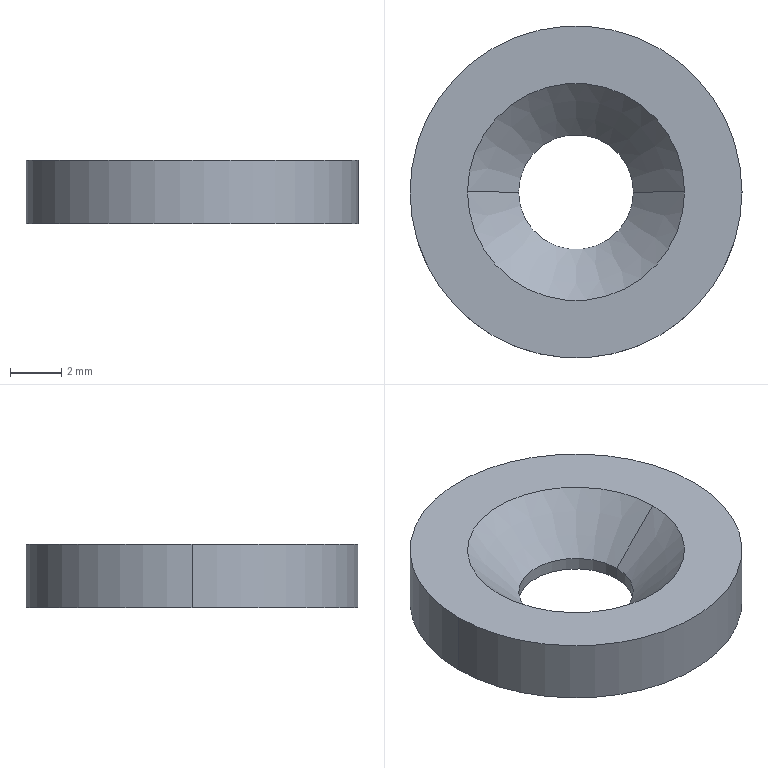Part | NX | features BREP 1 | 1 solid | 8 faces | box 13 x 13 x 2.5 mm | volume 255.418 mm3 | cylinder 4 | cone 2 | plane 2 | commonest cylinder face diameters 4.5 x2 13 x2
STEP:
#1=CARTESIAN_POINT('',(-4.25,0.,2.5));
#2=VERTEX_POINT('',#1);
#3=CARTESIAN_POINT('',(-2.25,0.,0.5));
#4=VERTEX_POINT('',#3);
#5=CARTESIAN_POINT('',(-4.25,0.,2.5));
#6=DIRECTION('',(-0.7071,0.,0.7071));
#7=VECTOR('',#6,1000.);
#8=LINE('',#5,#7);
#9=EDGE_CURVE('',#2,#4,#8,.F.);
#10=ORIENTED_EDGE('',*,*,#9,.T.);
#11=CARTESIAN_POINT('',(2.25,0.,0.5));
#12=VERTEX_POINT('',#11);
#13=CARTESIAN_POINT('',(0.,0.,0.5));
#14=DIRECTION('',(0.,0.,1.));
#15=DIRECTION('',(1.,0.,0.));
#16=AXIS2_PLACEMENT_3D('',#13,#14,#15);
#17=CIRCLE('',#16,2.25);
#18=EDGE_CURVE('',#12,#4,#17,.T.);
#19=ORIENTED_EDGE('',*,*,#18,.F.);
#20=CARTESIAN_POINT('',(4.25,0.,2.5));
#21=VERTEX_POINT('',#20);
#22=CARTESIAN_POINT('',(4.25,0.,2.5));
#23=DIRECTION('',(0.7071,0.,0.7071));
#24=VECTOR('',#23,1000.);
#25=LINE('',#22,#24);
#26=EDGE_CURVE('',#21,#12,#25,.F.);
#27=ORIENTED_EDGE('',*,*,#26,.F.);
#28=CARTESIAN_POINT('',(0.,0.,2.5));
#29=DIRECTION('',(0.,0.,1.));
#30=DIRECTION('',(1.,0.,0.));
#31=AXIS2_PLACEMENT_3D('',#28,#29,#30);
#32=CIRCLE('',#31,4.25);
#33=EDGE_CURVE('',#21,#2,#32,.T.);
#34=ORIENTED_EDGE('',*,*,#33,.T.);
#35=EDGE_LOOP('',(#10,#19,#27,#34));
#36=FACE_BOUND('',#35,.T.);
#37=CARTESIAN_POINT('',(0.,0.,2.5));
#38=DIRECTION('',(0.,0.,1.));
#39=DIRECTION('',(1.,0.,0.));
#40=AXIS2_PLACEMENT_3D('',#37,#38,#39);
#41=CONICAL_SURFACE('',#40,4.25,0.7854);
#42=ADVANCED_FACE('',(#36),#41,.F.);
#43=CARTESIAN_POINT('',(-2.25,0.,0.));
#44=VERTEX_POINT('',#43);
#45=CARTESIAN_POINT('',(-2.25,0.,2.5));
#46=DIRECTION('',(0.,0.,1.));
#47=VECTOR('',#46,1000.);
#48=LINE('',#45,#47);
#49=EDGE_CURVE('',#4,#44,#48,.F.);
#50=ORIENTED_EDGE('',*,*,#49,.T.);
#51=CARTESIAN_POINT('',(2.25,0.,0.));
#52=VERTEX_POINT('',#51);
#53=CARTESIAN_POINT('',(0.,0.,0.));
#54=DIRECTION('',(0.,0.,1.));
#55=DIRECTION('',(1.,0.,0.));
#56=AXIS2_PLACEMENT_3D('',#53,#54,#55);
#57=CIRCLE('',#56,2.25);
#58=EDGE_CURVE('',#52,#44,#57,.T.);
#59=ORIENTED_EDGE('',*,*,#58,.F.);
#60=CARTESIAN_POINT('',(2.25,0.,2.5));
#61=DIRECTION('',(0.,0.,1.));
#62=VECTOR('',#61,1000.);
#63=LINE('',#60,#62);
#64=EDGE_CURVE('',#12,#52,#63,.F.);
#65=ORIENTED_EDGE('',*,*,#64,.F.);
#66=ORIENTED_EDGE('',*,*,#18,.T.);
#67=EDGE_LOOP('',(#50,#59,#65,#66));
#68=FACE_BOUND('',#67,.T.);
#69=CARTESIAN_POINT('',(0.,0.,2.5));
#70=DIRECTION('',(0.,0.,1.));
#71=DIRECTION('',(1.,0.,0.));
#72=AXIS2_PLACEMENT_3D('',#69,#70,#71);
#73=CYLINDRICAL_SURFACE('',#72,2.25);
#74=ADVANCED_FACE('',(#68),#73,.F.);
#75=CARTESIAN_POINT('',(-6.5,0.,0.));
#76=VERTEX_POINT('',#75);
#77=CARTESIAN_POINT('',(6.5,0.,0.));
#78=VERTEX_POINT('',#77);
#79=CARTESIAN_POINT('',(0.,0.,0.));
#80=DIRECTION('',(0.,0.,1.));
#81=DIRECTION('',(1.,0.,0.));
#82=AXIS2_PLACEMENT_3D('',#79,#80,#81);
#83=CIRCLE('',#82,6.5);
#84=EDGE_CURVE('',#76,#78,#83,.T.);
#85=ORIENTED_EDGE('',*,*,#84,.F.);
#86=CARTESIAN_POINT('',(0.,0.,0.));
#87=DIRECTION('',(0.,0.,1.));
#88=DIRECTION('',(1.,0.,0.));
#89=AXIS2_PLACEMENT_3D('',#86,#87,#88);
#90=CIRCLE('',#89,6.5);
#91=EDGE_CURVE('',#78,#76,#90,.T.);
#92=ORIENTED_EDGE('',*,*,#91,.F.);
#93=EDGE_LOOP('',(#85,#92));
#94=FACE_BOUND('',#93,.T.);
#95=ORIENTED_EDGE('',*,*,#58,.T.);
#96=CARTESIAN_POINT('',(0.,0.,0.));
#97=DIRECTION('',(0.,0.,1.));
#98=DIRECTION('',(1.,0.,0.));
#99=AXIS2_PLACEMENT_3D('',#96,#97,#98);
#100=CIRCLE('',#99,2.25);
#101=EDGE_CURVE('',#44,#52,#100,.T.);
#102=ORIENTED_EDGE('',*,*,#101,.T.);
#103=EDGE_LOOP('',(#95,#102));
#104=FACE_BOUND('',#103,.T.);
#105=CARTESIAN_POINT('',(0.,0.,0.));
#106=DIRECTION('',(0.,0.,1.));
#107=DIRECTION('',(1.,0.,0.));
#108=AXIS2_PLACEMENT_3D('',#105,#106,#107);
#109=PLANE('',#108);
#110=ADVANCED_FACE('',(#94,#104),#109,.F.);
#111=CARTESIAN_POINT('',(-6.5,0.,2.5));
#112=VERTEX_POINT('',#111);
#113=CARTESIAN_POINT('',(6.5,0.,2.5));
#114=VERTEX_POINT('',#113);
#115=CARTESIAN_POINT('',(0.,0.,2.5));
#116=DIRECTION('',(0.,0.,1.));
#117=DIRECTION('',(1.,0.,0.));
#118=AXIS2_PLACEMENT_3D('',#115,#116,#117);
#119=CIRCLE('',#118,6.5);
#120=EDGE_CURVE('',#112,#114,#119,.T.);
#121=ORIENTED_EDGE('',*,*,#120,.T.);
#122=CARTESIAN_POINT('',(0.,0.,2.5));
#123=DIRECTION('',(0.,0.,1.));
#124=DIRECTION('',(1.,0.,0.));
#125=AXIS2_PLACEMENT_3D('',#122,#123,#124);
#126=CIRCLE('',#125,6.5);
#127=EDGE_CURVE('',#114,#112,#126,.T.);
#128=ORIENTED_EDGE('',*,*,#127,.T.);
#129=EDGE_LOOP('',(#121,#128));
#130=FACE_BOUND('',#129,.T.);
#131=ORIENTED_EDGE('',*,*,#33,.F.);
#132=CARTESIAN_POINT('',(0.,0.,2.5));
#133=DIRECTION('',(0.,0.,1.));
#134=DIRECTION('',(1.,0.,0.));
#135=AXIS2_PLACEMENT_3D('',#132,#133,#134);
#136=CIRCLE('',#135,4.25);
#137=EDGE_CURVE('',#2,#21,#136,.T.);
#138=ORIENTED_EDGE('',*,*,#137,.F.);
#139=EDGE_LOOP('',(#131,#138));
#140=FACE_BOUND('',#139,.T.);
#141=CARTESIAN_POINT('',(0.,0.,2.5));
#142=DIRECTION('',(0.,0.,1.));
#143=DIRECTION('',(1.,0.,0.));
#144=AXIS2_PLACEMENT_3D('',#141,#142,#143);
#145=PLANE('',#144);
#146=ADVANCED_FACE('',(#130,#140),#145,.T.);
#147=CARTESIAN_POINT('',(6.5,0.,2.5));
#148=DIRECTION('',(0.,0.,-1.));
#149=VECTOR('',#148,1000.);
#150=LINE('',#147,#149);
#151=EDGE_CURVE('',#114,#78,#150,.T.);
#152=ORIENTED_EDGE('',*,*,#151,.F.);
#153=ORIENTED_EDGE('',*,*,#120,.F.);
#154=CARTESIAN_POINT('',(-6.5,0.,2.5));
#155=DIRECTION('',(0.,0.,-1.));
#156=VECTOR('',#155,1000.);
#157=LINE('',#154,#156);
#158=EDGE_CURVE('',#112,#76,#157,.T.);
#159=ORIENTED_EDGE('',*,*,#158,.T.);
#160=ORIENTED_EDGE('',*,*,#84,.T.);
#161=EDGE_LOOP('',(#152,#153,#159,#160));
#162=FACE_BOUND('',#161,.T.);
#163=CARTESIAN_POINT('',(0.,0.,2.5));
#164=DIRECTION('',(0.,0.,-1.));
#165=DIRECTION('',(-1.,0.,0.));
#166=AXIS2_PLACEMENT_3D('',#163,#164,#165);
#167=CYLINDRICAL_SURFACE('',#166,6.5);
#168=ADVANCED_FACE('',(#162),#167,.T.);
#169=ORIENTED_EDGE('',*,*,#127,.F.);
#170=ORIENTED_EDGE('',*,*,#151,.T.);
#171=ORIENTED_EDGE('',*,*,#91,.T.);
#172=ORIENTED_EDGE('',*,*,#158,.F.);
#173=EDGE_LOOP('',(#169,#170,#171,#172));
#174=FACE_BOUND('',#173,.T.);
#175=CARTESIAN_POINT('',(0.,0.,2.5));
#176=DIRECTION('',(0.,0.,-1.));
#177=DIRECTION('',(-1.,0.,0.));
#178=AXIS2_PLACEMENT_3D('',#175,#176,#177);
#179=CYLINDRICAL_SURFACE('',#178,6.5);
#180=ADVANCED_FACE('',(#174),#179,.T.);
#181=ORIENTED_EDGE('',*,*,#101,.F.);
#182=ORIENTED_EDGE('',*,*,#49,.F.);
#183=CARTESIAN_POINT('',(0.,0.,0.5));
#184=DIRECTION('',(0.,0.,1.));
#185=DIRECTION('',(1.,0.,0.));
#186=AXIS2_PLACEMENT_3D('',#183,#184,#185);
#187=CIRCLE('',#186,2.25);
#188=EDGE_CURVE('',#4,#12,#187,.T.);
#189=ORIENTED_EDGE('',*,*,#188,.T.);
#190=ORIENTED_EDGE('',*,*,#64,.T.);
#191=EDGE_LOOP('',(#181,#182,#189,#190));
#192=FACE_BOUND('',#191,.T.);
#193=CARTESIAN_POINT('',(0.,0.,2.5));
#194=DIRECTION('',(0.,0.,1.));
#195=DIRECTION('',(1.,0.,0.));
#196=AXIS2_PLACEMENT_3D('',#193,#194,#195);
#197=CYLINDRICAL_SURFACE('',#196,2.25);
#198=ADVANCED_FACE('',(#192),#197,.F.);
#199=ORIENTED_EDGE('',*,*,#188,.F.);
#200=ORIENTED_EDGE('',*,*,#9,.F.);
#201=ORIENTED_EDGE('',*,*,#137,.T.);
#202=ORIENTED_EDGE('',*,*,#26,.T.);
#203=EDGE_LOOP('',(#199,#200,#201,#202));
#204=FACE_BOUND('',#203,.T.);
#205=CARTESIAN_POINT('',(0.,0.,2.5));
#206=DIRECTION('',(0.,0.,1.));
#207=DIRECTION('',(1.,0.,0.));
#208=AXIS2_PLACEMENT_3D('',#205,#206,#207);
#209=CONICAL_SURFACE('',#208,4.25,0.7854);
#210=ADVANCED_FACE('',(#204),#209,.F.);
#211=CLOSED_SHELL('',(#42,#74,#110,#146,#168,#180,#198,#210));
#212=MANIFOLD_SOLID_BREP('',#211);
#213=(LENGTH_UNIT()NAMED_UNIT(*)SI_UNIT(.MILLI.,.METRE.));
#214=UNCERTAINTY_MEASURE_WITH_UNIT(LENGTH_MEASURE(0.00001),#213,'','');
#215=(NAMED_UNIT(*)PLANE_ANGLE_UNIT()SI_UNIT($,.RADIAN.));
#216=(NAMED_UNIT(*)SI_UNIT($,.STERADIAN.)SOLID_ANGLE_UNIT());
#217=(GEOMETRIC_REPRESENTATION_CONTEXT(3)GLOBAL_UNCERTAINTY_ASSIGNED_CONTEXT((#214))GLOBAL_UNIT_ASSIGNED_CONTEXT((#213,#215,#216))REPRESENTATION_CONTEXT('',''));
#218=ADVANCED_BREP_SHAPE_REPRESENTATION('',(#212),#217);